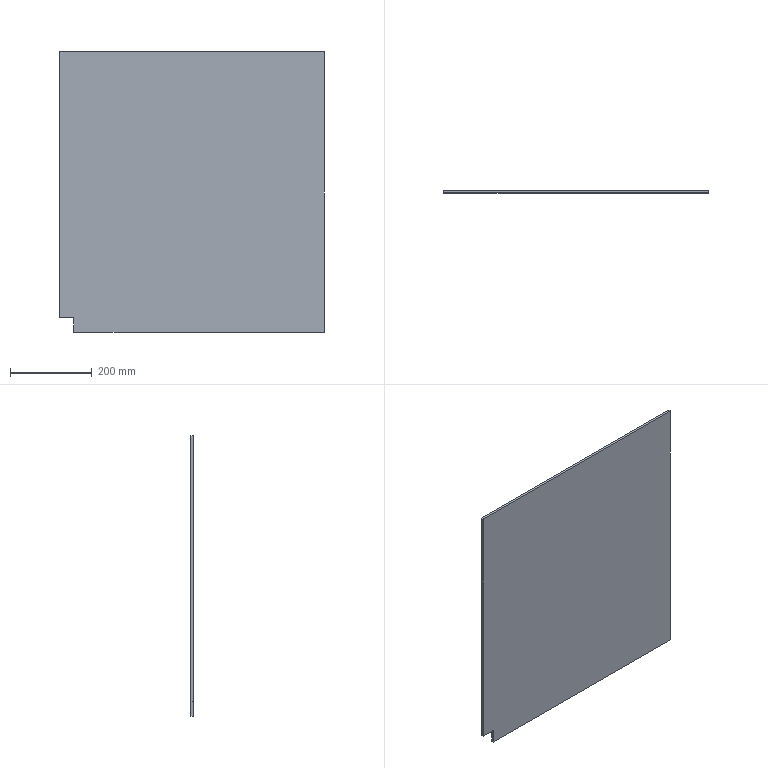Part | SolidWorks | features BaseBody 1, ICE 1 | 1 solid | 8 faces | box 647 x 5 x 685 mm | volume 2209850 mm3 | plane 8
STEP:
#1=CARTESIAN_POINT('',(87.,605.,-360.));
#2=VERTEX_POINT('',#1);
#3=CARTESIAN_POINT('',(87.,605.,325.));
#4=VERTEX_POINT('',#3);
#5=CARTESIAN_POINT('',(87.,605.,-360.));
#6=DIRECTION('',(0.,0.,1.));
#7=VECTOR('',#6,1000.);
#8=LINE('',#5,#7);
#9=EDGE_CURVE('',#2,#4,#8,.T.);
#10=ORIENTED_EDGE('',*,*,#9,.F.);
#11=CARTESIAN_POINT('',(-525.,605.,-360.));
#12=VERTEX_POINT('',#11);
#13=CARTESIAN_POINT('',(-525.,605.,-360.));
#14=DIRECTION('',(1.,0.,0.));
#15=VECTOR('',#14,1000.);
#16=LINE('',#13,#15);
#17=EDGE_CURVE('',#12,#2,#16,.T.);
#18=ORIENTED_EDGE('',*,*,#17,.F.);
#19=CARTESIAN_POINT('',(-525.,605.,-325.));
#20=VERTEX_POINT('',#19);
#21=CARTESIAN_POINT('',(-525.,605.,-325.));
#22=DIRECTION('',(0.,0.,-1.));
#23=VECTOR('',#22,1000.);
#24=LINE('',#21,#23);
#25=EDGE_CURVE('',#20,#12,#24,.T.);
#26=ORIENTED_EDGE('',*,*,#25,.F.);
#27=CARTESIAN_POINT('',(-560.,605.,-325.));
#28=VERTEX_POINT('',#27);
#29=CARTESIAN_POINT('',(-560.,605.,-325.));
#30=DIRECTION('',(1.,0.,0.));
#31=VECTOR('',#30,1000.);
#32=LINE('',#29,#31);
#33=EDGE_CURVE('',#28,#20,#32,.T.);
#34=ORIENTED_EDGE('',*,*,#33,.F.);
#35=CARTESIAN_POINT('',(-560.,605.,325.));
#36=VERTEX_POINT('',#35);
#37=CARTESIAN_POINT('',(-560.,605.,325.));
#38=DIRECTION('',(0.,0.,-1.));
#39=VECTOR('',#38,1000.);
#40=LINE('',#37,#39);
#41=EDGE_CURVE('',#36,#28,#40,.T.);
#42=ORIENTED_EDGE('',*,*,#41,.F.);
#43=CARTESIAN_POINT('',(560.,605.,325.));
#44=DIRECTION('',(-1.,0.,0.));
#45=VECTOR('',#44,1000.);
#46=LINE('',#43,#45);
#47=EDGE_CURVE('',#4,#36,#46,.T.);
#48=ORIENTED_EDGE('',*,*,#47,.F.);
#49=EDGE_LOOP('',(#10,#18,#26,#34,#42,#48));
#50=FACE_OUTER_BOUND('',#49,.T.);
#51=CARTESIAN_POINT('',(0.,605.,-17.5));
#52=DIRECTION('',(0.,1.,0.));
#53=DIRECTION('',(1.,0.,0.));
#54=AXIS2_PLACEMENT_3D('',#51,#52,#53);
#55=PLANE('',#54);
#56=ADVANCED_FACE('',(#50),#55,.T.);
#57=CARTESIAN_POINT('',(87.,600.,325.));
#58=VERTEX_POINT('',#57);
#59=CARTESIAN_POINT('',(87.,600.,-360.));
#60=VERTEX_POINT('',#59);
#61=CARTESIAN_POINT('',(87.,600.,-17.5));
#62=DIRECTION('',(0.,0.,-1.));
#63=VECTOR('',#62,1000.);
#64=LINE('',#61,#63);
#65=EDGE_CURVE('',#58,#60,#64,.T.);
#66=ORIENTED_EDGE('',*,*,#65,.F.);
#67=CARTESIAN_POINT('',(-560.,600.,325.));
#68=VERTEX_POINT('',#67);
#69=CARTESIAN_POINT('',(-560.,600.,325.));
#70=DIRECTION('',(1.,0.,0.));
#71=VECTOR('',#70,1000.);
#72=LINE('',#69,#71);
#73=EDGE_CURVE('',#68,#58,#72,.T.);
#74=ORIENTED_EDGE('',*,*,#73,.F.);
#75=CARTESIAN_POINT('',(-560.,600.,-325.));
#76=VERTEX_POINT('',#75);
#77=CARTESIAN_POINT('',(-560.,600.,-325.));
#78=DIRECTION('',(0.,0.,1.));
#79=VECTOR('',#78,1000.);
#80=LINE('',#77,#79);
#81=EDGE_CURVE('',#76,#68,#80,.T.);
#82=ORIENTED_EDGE('',*,*,#81,.F.);
#83=CARTESIAN_POINT('',(-525.,600.,-325.));
#84=VERTEX_POINT('',#83);
#85=CARTESIAN_POINT('',(-525.,600.,-325.));
#86=DIRECTION('',(-1.,0.,0.));
#87=VECTOR('',#86,1000.);
#88=LINE('',#85,#87);
#89=EDGE_CURVE('',#84,#76,#88,.T.);
#90=ORIENTED_EDGE('',*,*,#89,.F.);
#91=CARTESIAN_POINT('',(-525.,600.,-360.));
#92=VERTEX_POINT('',#91);
#93=CARTESIAN_POINT('',(-525.,600.,-360.));
#94=DIRECTION('',(0.,0.,1.));
#95=VECTOR('',#94,1000.);
#96=LINE('',#93,#95);
#97=EDGE_CURVE('',#92,#84,#96,.T.);
#98=ORIENTED_EDGE('',*,*,#97,.F.);
#99=CARTESIAN_POINT('',(560.,600.,-360.));
#100=DIRECTION('',(-1.,0.,0.));
#101=VECTOR('',#100,1000.);
#102=LINE('',#99,#101);
#103=EDGE_CURVE('',#60,#92,#102,.T.);
#104=ORIENTED_EDGE('',*,*,#103,.F.);
#105=EDGE_LOOP('',(#66,#74,#82,#90,#98,#104));
#106=FACE_OUTER_BOUND('',#105,.T.);
#107=CARTESIAN_POINT('',(0.,600.,-17.5));
#108=DIRECTION('',(0.,-1.,0.));
#109=DIRECTION('',(0.,0.,-1.));
#110=AXIS2_PLACEMENT_3D('',#107,#108,#109);
#111=PLANE('',#110);
#112=ADVANCED_FACE('',(#106),#111,.T.);
#113=ORIENTED_EDGE('',*,*,#33,.T.);
#114=CARTESIAN_POINT('',(-525.,600.,-325.));
#115=DIRECTION('',(0.,1.,0.));
#116=VECTOR('',#115,1000.);
#117=LINE('',#114,#116);
#118=EDGE_CURVE('',#84,#20,#117,.T.);
#119=ORIENTED_EDGE('',*,*,#118,.F.);
#120=ORIENTED_EDGE('',*,*,#89,.T.);
#121=CARTESIAN_POINT('',(-560.,605.,-325.));
#122=DIRECTION('',(0.,-1.,0.));
#123=VECTOR('',#122,1000.);
#124=LINE('',#121,#123);
#125=EDGE_CURVE('',#28,#76,#124,.T.);
#126=ORIENTED_EDGE('',*,*,#125,.F.);
#127=EDGE_LOOP('',(#113,#119,#120,#126));
#128=FACE_OUTER_BOUND('',#127,.T.);
#129=CARTESIAN_POINT('',(-560.,605.,-325.));
#130=DIRECTION('',(0.,0.,-1.));
#131=DIRECTION('',(0.,-1.,0.));
#132=AXIS2_PLACEMENT_3D('',#129,#130,#131);
#133=PLANE('',#132);
#134=ADVANCED_FACE('',(#128),#133,.T.);
#135=ORIENTED_EDGE('',*,*,#25,.T.);
#136=CARTESIAN_POINT('',(-525.,600.,-360.));
#137=DIRECTION('',(0.,1.,0.));
#138=VECTOR('',#137,1000.);
#139=LINE('',#136,#138);
#140=EDGE_CURVE('',#92,#12,#139,.T.);
#141=ORIENTED_EDGE('',*,*,#140,.F.);
#142=ORIENTED_EDGE('',*,*,#97,.T.);
#143=ORIENTED_EDGE('',*,*,#118,.T.);
#144=EDGE_LOOP('',(#135,#141,#142,#143));
#145=FACE_OUTER_BOUND('',#144,.T.);
#146=CARTESIAN_POINT('',(-525.,605.,-325.));
#147=DIRECTION('',(-1.,0.,0.));
#148=DIRECTION('',(0.,0.,1.));
#149=AXIS2_PLACEMENT_3D('',#146,#147,#148);
#150=PLANE('',#149);
#151=ADVANCED_FACE('',(#145),#150,.T.);
#152=CARTESIAN_POINT('',(87.,595.,-360.));
#153=DIRECTION('',(0.,1.,0.));
#154=VECTOR('',#153,1000.);
#155=LINE('',#152,#154);
#156=EDGE_CURVE('',#60,#2,#155,.T.);
#157=ORIENTED_EDGE('',*,*,#156,.F.);
#158=ORIENTED_EDGE('',*,*,#103,.T.);
#159=ORIENTED_EDGE('',*,*,#140,.T.);
#160=ORIENTED_EDGE('',*,*,#17,.T.);
#161=EDGE_LOOP('',(#157,#158,#159,#160));
#162=FACE_OUTER_BOUND('',#161,.T.);
#163=CARTESIAN_POINT('',(-525.,605.,-360.));
#164=DIRECTION('',(0.,0.,-1.));
#165=DIRECTION('',(-1.,0.,0.));
#166=AXIS2_PLACEMENT_3D('',#163,#164,#165);
#167=PLANE('',#166);
#168=ADVANCED_FACE('',(#162),#167,.T.);
#169=CARTESIAN_POINT('',(87.,605.,325.));
#170=DIRECTION('',(0.,-1.,0.));
#171=VECTOR('',#170,1000.);
#172=LINE('',#169,#171);
#173=EDGE_CURVE('',#4,#58,#172,.T.);
#174=ORIENTED_EDGE('',*,*,#173,.F.);
#175=ORIENTED_EDGE('',*,*,#47,.T.);
#176=CARTESIAN_POINT('',(-560.,600.,325.));
#177=DIRECTION('',(0.,1.,0.));
#178=VECTOR('',#177,1000.);
#179=LINE('',#176,#178);
#180=EDGE_CURVE('',#68,#36,#179,.T.);
#181=ORIENTED_EDGE('',*,*,#180,.F.);
#182=ORIENTED_EDGE('',*,*,#73,.T.);
#183=EDGE_LOOP('',(#174,#175,#181,#182));
#184=FACE_OUTER_BOUND('',#183,.T.);
#185=CARTESIAN_POINT('',(560.,605.,325.));
#186=DIRECTION('',(0.,0.,1.));
#187=DIRECTION('',(1.,0.,0.));
#188=AXIS2_PLACEMENT_3D('',#185,#186,#187);
#189=PLANE('',#188);
#190=ADVANCED_FACE('',(#184),#189,.T.);
#191=ORIENTED_EDGE('',*,*,#41,.T.);
#192=ORIENTED_EDGE('',*,*,#125,.T.);
#193=ORIENTED_EDGE('',*,*,#81,.T.);
#194=ORIENTED_EDGE('',*,*,#180,.T.);
#195=EDGE_LOOP('',(#191,#192,#193,#194));
#196=FACE_OUTER_BOUND('',#195,.T.);
#197=CARTESIAN_POINT('',(-560.,605.,325.));
#198=DIRECTION('',(-1.,0.,0.));
#199=DIRECTION('',(0.,0.,1.));
#200=AXIS2_PLACEMENT_3D('',#197,#198,#199);
#201=PLANE('',#200);
#202=ADVANCED_FACE('',(#196),#201,.T.);
#203=ORIENTED_EDGE('',*,*,#65,.T.);
#204=ORIENTED_EDGE('',*,*,#156,.T.);
#205=ORIENTED_EDGE('',*,*,#9,.T.);
#206=ORIENTED_EDGE('',*,*,#173,.T.);
#207=EDGE_LOOP('',(#203,#204,#205,#206));
#208=FACE_OUTER_BOUND('',#207,.T.);
#209=CARTESIAN_POINT('',(87.,595.,-360.));
#210=DIRECTION('',(-1.,0.,0.));
#211=DIRECTION('',(0.,0.,1.));
#212=AXIS2_PLACEMENT_3D('',#209,#210,#211);
#213=PLANE('',#212);
#214=ADVANCED_FACE('',(#208),#213,.F.);
#215=CLOSED_SHELL('',(#56,#112,#134,#151,#168,#190,#202,#214));
#216=MANIFOLD_SOLID_BREP('',#215);
#217=CARTESIAN_POINT('',(0.,0.,0.));
#218=DIRECTION('',(0.,0.,1.));
#219=DIRECTION('',(1.,0.,0.));
#220=AXIS2_PLACEMENT_3D('',#217,#218,#219);
#221=(LENGTH_UNIT()NAMED_UNIT(*)SI_UNIT(.MILLI.,.METRE.));
#222=UNCERTAINTY_MEASURE_WITH_UNIT(LENGTH_MEASURE(0.00001),#221,'','');
#223=(NAMED_UNIT(*)PLANE_ANGLE_UNIT()SI_UNIT($,.RADIAN.));
#224=(NAMED_UNIT(*)SI_UNIT($,.STERADIAN.)SOLID_ANGLE_UNIT());
#225=(GEOMETRIC_REPRESENTATION_CONTEXT(3)GLOBAL_UNCERTAINTY_ASSIGNED_CONTEXT((#222))GLOBAL_UNIT_ASSIGNED_CONTEXT((#221,#223,#224))REPRESENTATION_CONTEXT('',''));
#226=ADVANCED_BREP_SHAPE_REPRESENTATION('',(#216,#220),#225);